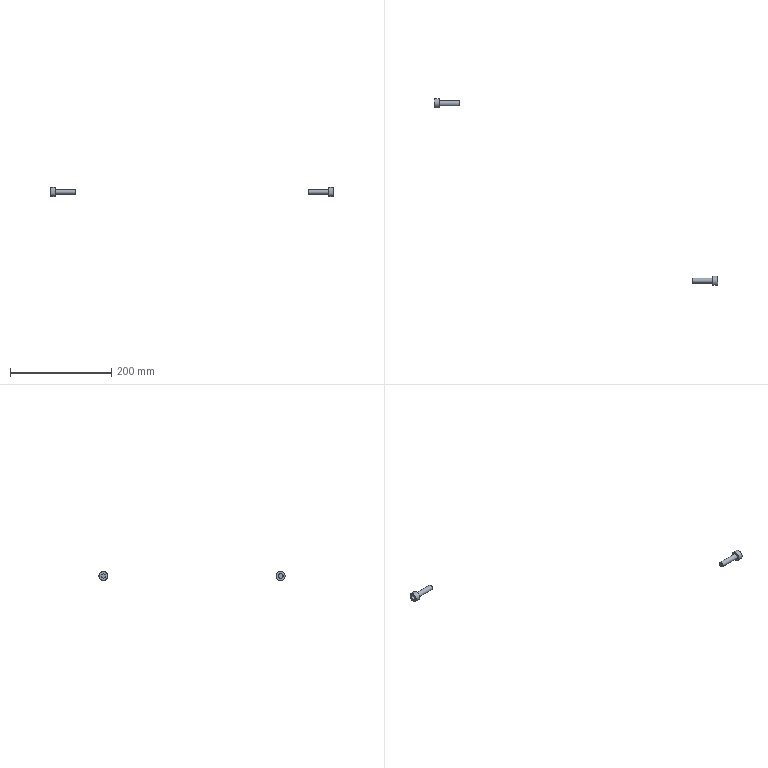Part | STEP file | M10.00-20 | 2 solids | 28 faces | box 560 x 368 x 18 mm | volume 10650 mm3 | plane 20 | cylinder 4 | cone 4 | commonest cylinder face diameters 10 x2 18 x2